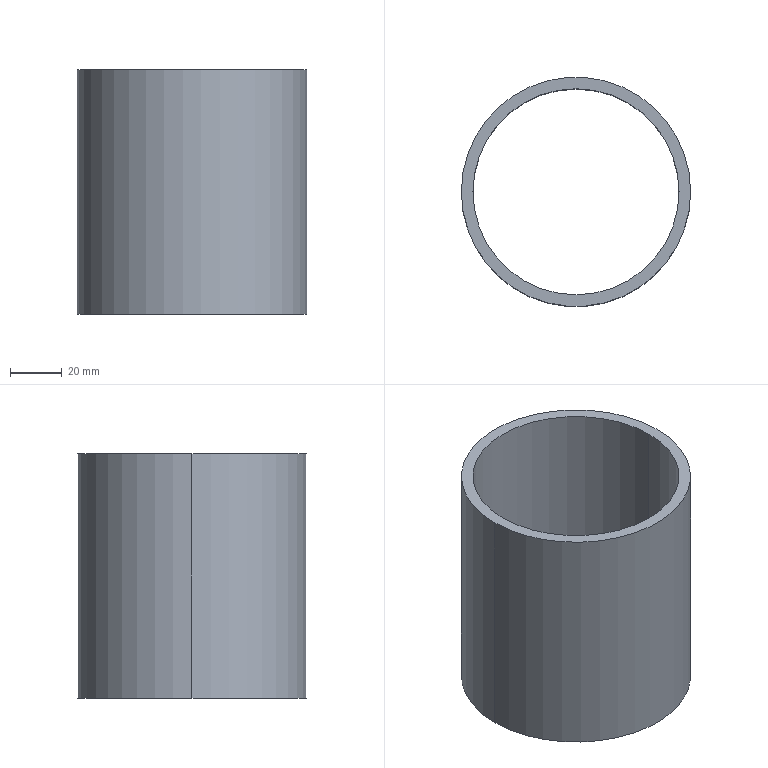Part | SolidWorks | features BaseBody 1 | 1 solid | 6 faces | box 89 x 89 x 95 mm | volume 113486 mm3 | cylinder 4 | plane 2 | commonest cylinder face diameters 80 x2 89 x2
STEP:
#1=CARTESIAN_POINT('',(-40.,0.,95.));
#2=VERTEX_POINT('',#1);
#3=CARTESIAN_POINT('',(40.,0.,95.));
#4=VERTEX_POINT('',#3);
#5=CARTESIAN_POINT('',(0.,0.,95.));
#6=DIRECTION('',(0.,0.,1.));
#7=DIRECTION('',(1.,0.,0.));
#8=AXIS2_PLACEMENT_3D('',#5,#6,#7);
#9=CIRCLE('',#8,40.);
#10=EDGE_CURVE('',#2,#4,#9,.T.);
#11=ORIENTED_EDGE('',*,*,#10,.T.);
#12=CARTESIAN_POINT('',(40.,0.,0.));
#13=VERTEX_POINT('',#12);
#14=CARTESIAN_POINT('',(40.,0.,95.));
#15=DIRECTION('',(0.,0.,-1.));
#16=VECTOR('',#15,1000.);
#17=LINE('',#14,#16);
#18=EDGE_CURVE('',#4,#13,#17,.T.);
#19=ORIENTED_EDGE('',*,*,#18,.T.);
#20=CARTESIAN_POINT('',(-40.,0.,0.));
#21=VERTEX_POINT('',#20);
#22=CARTESIAN_POINT('',(0.,0.,0.));
#23=DIRECTION('',(0.,0.,1.));
#24=DIRECTION('',(1.,0.,0.));
#25=AXIS2_PLACEMENT_3D('',#22,#23,#24);
#26=CIRCLE('',#25,40.);
#27=EDGE_CURVE('',#21,#13,#26,.T.);
#28=ORIENTED_EDGE('',*,*,#27,.F.);
#29=CARTESIAN_POINT('',(-40.,0.,95.));
#30=DIRECTION('',(0.,0.,-1.));
#31=VECTOR('',#30,1000.);
#32=LINE('',#29,#31);
#33=EDGE_CURVE('',#2,#21,#32,.T.);
#34=ORIENTED_EDGE('',*,*,#33,.F.);
#35=EDGE_LOOP('',(#11,#19,#28,#34));
#36=FACE_OUTER_BOUND('',#35,.T.);
#37=CARTESIAN_POINT('',(0.,0.,95.));
#38=DIRECTION('',(0.,0.,-1.));
#39=DIRECTION('',(-1.,0.,0.));
#40=AXIS2_PLACEMENT_3D('',#37,#38,#39);
#41=CYLINDRICAL_SURFACE('',#40,40.);
#42=ADVANCED_FACE('',(#36),#41,.F.);
#43=CARTESIAN_POINT('',(44.5,0.,95.));
#44=VERTEX_POINT('',#43);
#45=CARTESIAN_POINT('',(-44.5,0.,95.));
#46=VERTEX_POINT('',#45);
#47=CARTESIAN_POINT('',(0.,0.,95.));
#48=DIRECTION('',(0.,0.,1.));
#49=DIRECTION('',(1.,0.,0.));
#50=AXIS2_PLACEMENT_3D('',#47,#48,#49);
#51=CIRCLE('',#50,44.5);
#52=EDGE_CURVE('',#44,#46,#51,.T.);
#53=ORIENTED_EDGE('',*,*,#52,.F.);
#54=CARTESIAN_POINT('',(44.5,0.,0.));
#55=VERTEX_POINT('',#54);
#56=CARTESIAN_POINT('',(44.5,0.,95.));
#57=DIRECTION('',(0.,0.,-1.));
#58=VECTOR('',#57,1000.);
#59=LINE('',#56,#58);
#60=EDGE_CURVE('',#44,#55,#59,.T.);
#61=ORIENTED_EDGE('',*,*,#60,.T.);
#62=CARTESIAN_POINT('',(-44.5,0.,0.));
#63=VERTEX_POINT('',#62);
#64=CARTESIAN_POINT('',(0.,0.,0.));
#65=DIRECTION('',(0.,0.,1.));
#66=DIRECTION('',(1.,0.,0.));
#67=AXIS2_PLACEMENT_3D('',#64,#65,#66);
#68=CIRCLE('',#67,44.5);
#69=EDGE_CURVE('',#55,#63,#68,.T.);
#70=ORIENTED_EDGE('',*,*,#69,.T.);
#71=CARTESIAN_POINT('',(-44.5,0.,95.));
#72=DIRECTION('',(0.,0.,-1.));
#73=VECTOR('',#72,1000.);
#74=LINE('',#71,#73);
#75=EDGE_CURVE('',#46,#63,#74,.T.);
#76=ORIENTED_EDGE('',*,*,#75,.F.);
#77=EDGE_LOOP('',(#53,#61,#70,#76));
#78=FACE_OUTER_BOUND('',#77,.T.);
#79=CARTESIAN_POINT('',(0.,0.,95.));
#80=DIRECTION('',(0.,0.,-1.));
#81=DIRECTION('',(-1.,0.,0.));
#82=AXIS2_PLACEMENT_3D('',#79,#80,#81);
#83=CYLINDRICAL_SURFACE('',#82,44.5);
#84=ADVANCED_FACE('',(#78),#83,.T.);
#85=CARTESIAN_POINT('',(0.,0.,95.));
#86=DIRECTION('',(0.,0.,1.));
#87=DIRECTION('',(1.,0.,0.));
#88=AXIS2_PLACEMENT_3D('',#85,#86,#87);
#89=CIRCLE('',#88,44.5);
#90=EDGE_CURVE('',#46,#44,#89,.T.);
#91=ORIENTED_EDGE('',*,*,#90,.T.);
#92=ORIENTED_EDGE('',*,*,#52,.T.);
#93=EDGE_LOOP('',(#91,#92));
#94=FACE_OUTER_BOUND('',#93,.T.);
#95=ORIENTED_EDGE('',*,*,#10,.F.);
#96=CARTESIAN_POINT('',(0.,0.,95.));
#97=DIRECTION('',(0.,0.,1.));
#98=DIRECTION('',(1.,0.,0.));
#99=AXIS2_PLACEMENT_3D('',#96,#97,#98);
#100=CIRCLE('',#99,40.);
#101=EDGE_CURVE('',#4,#2,#100,.T.);
#102=ORIENTED_EDGE('',*,*,#101,.F.);
#103=EDGE_LOOP('',(#95,#102));
#104=FACE_BOUND('',#103,.T.);
#105=CARTESIAN_POINT('',(0.,0.,95.));
#106=DIRECTION('',(0.,0.,1.));
#107=DIRECTION('',(1.,0.,0.));
#108=AXIS2_PLACEMENT_3D('',#105,#106,#107);
#109=PLANE('',#108);
#110=ADVANCED_FACE('',(#94,#104),#109,.T.);
#111=CARTESIAN_POINT('',(0.,0.,0.));
#112=DIRECTION('',(0.,0.,1.));
#113=DIRECTION('',(1.,0.,0.));
#114=AXIS2_PLACEMENT_3D('',#111,#112,#113);
#115=CIRCLE('',#114,44.5);
#116=EDGE_CURVE('',#63,#55,#115,.T.);
#117=ORIENTED_EDGE('',*,*,#116,.F.);
#118=ORIENTED_EDGE('',*,*,#69,.F.);
#119=EDGE_LOOP('',(#117,#118));
#120=FACE_OUTER_BOUND('',#119,.T.);
#121=ORIENTED_EDGE('',*,*,#27,.T.);
#122=CARTESIAN_POINT('',(0.,0.,0.));
#123=DIRECTION('',(0.,0.,1.));
#124=DIRECTION('',(1.,0.,0.));
#125=AXIS2_PLACEMENT_3D('',#122,#123,#124);
#126=CIRCLE('',#125,40.);
#127=EDGE_CURVE('',#13,#21,#126,.T.);
#128=ORIENTED_EDGE('',*,*,#127,.T.);
#129=EDGE_LOOP('',(#121,#128));
#130=FACE_BOUND('',#129,.T.);
#131=CARTESIAN_POINT('',(0.,0.,0.));
#132=DIRECTION('',(0.,0.,1.));
#133=DIRECTION('',(1.,0.,0.));
#134=AXIS2_PLACEMENT_3D('',#131,#132,#133);
#135=PLANE('',#134);
#136=ADVANCED_FACE('',(#120,#130),#135,.F.);
#137=ORIENTED_EDGE('',*,*,#60,.F.);
#138=ORIENTED_EDGE('',*,*,#90,.F.);
#139=ORIENTED_EDGE('',*,*,#75,.T.);
#140=ORIENTED_EDGE('',*,*,#116,.T.);
#141=EDGE_LOOP('',(#137,#138,#139,#140));
#142=FACE_OUTER_BOUND('',#141,.T.);
#143=CARTESIAN_POINT('',(0.,0.,95.));
#144=DIRECTION('',(0.,0.,-1.));
#145=DIRECTION('',(-1.,0.,0.));
#146=AXIS2_PLACEMENT_3D('',#143,#144,#145);
#147=CYLINDRICAL_SURFACE('',#146,44.5);
#148=ADVANCED_FACE('',(#142),#147,.T.);
#149=ORIENTED_EDGE('',*,*,#18,.F.);
#150=ORIENTED_EDGE('',*,*,#101,.T.);
#151=ORIENTED_EDGE('',*,*,#33,.T.);
#152=ORIENTED_EDGE('',*,*,#127,.F.);
#153=EDGE_LOOP('',(#149,#150,#151,#152));
#154=FACE_OUTER_BOUND('',#153,.T.);
#155=CARTESIAN_POINT('',(0.,0.,95.));
#156=DIRECTION('',(0.,0.,-1.));
#157=DIRECTION('',(-1.,0.,0.));
#158=AXIS2_PLACEMENT_3D('',#155,#156,#157);
#159=CYLINDRICAL_SURFACE('',#158,40.);
#160=ADVANCED_FACE('',(#154),#159,.F.);
#161=CLOSED_SHELL('',(#42,#84,#110,#136,#148,#160));
#162=MANIFOLD_SOLID_BREP('',#161);
#163=CARTESIAN_POINT('',(0.,0.,0.));
#164=DIRECTION('',(0.,0.,1.));
#165=DIRECTION('',(1.,0.,0.));
#166=AXIS2_PLACEMENT_3D('',#163,#164,#165);
#167=(LENGTH_UNIT()NAMED_UNIT(*)SI_UNIT(.MILLI.,.METRE.));
#168=UNCERTAINTY_MEASURE_WITH_UNIT(LENGTH_MEASURE(0.00001),#167,'','');
#169=(NAMED_UNIT(*)PLANE_ANGLE_UNIT()SI_UNIT($,.RADIAN.));
#170=(NAMED_UNIT(*)SI_UNIT($,.STERADIAN.)SOLID_ANGLE_UNIT());
#171=(GEOMETRIC_REPRESENTATION_CONTEXT(3)GLOBAL_UNCERTAINTY_ASSIGNED_CONTEXT((#168))GLOBAL_UNIT_ASSIGNED_CONTEXT((#167,#169,#170))REPRESENTATION_CONTEXT('',''));
#172=ADVANCED_BREP_SHAPE_REPRESENTATION('',(#162,#166),#171);